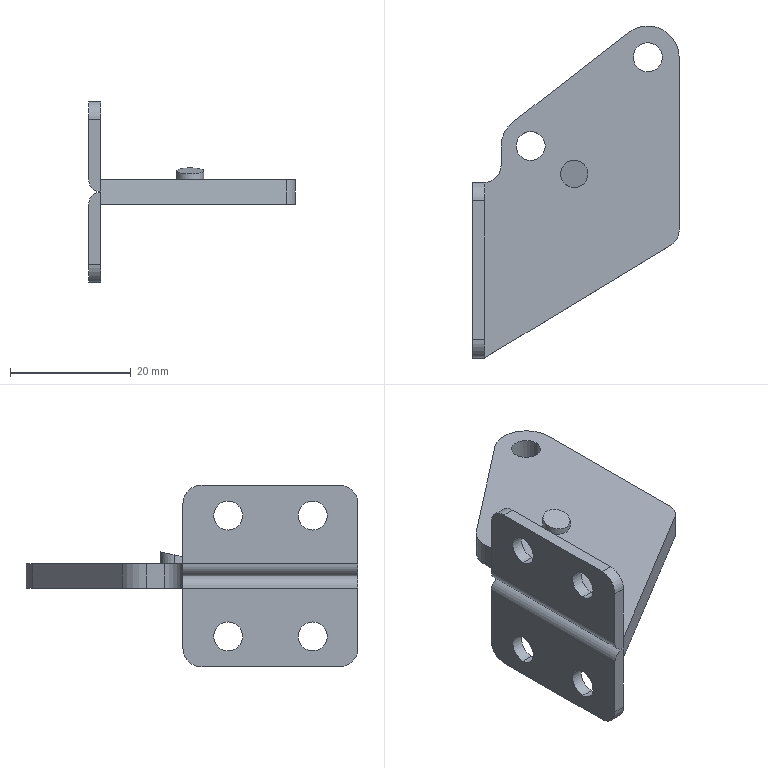Part | SolidWorks | features BaseBody 1 | 1 solid | 42 faces | box 34.2 x 55.001 x 30 mm | volume 6148 mm3 | cylinder 24 | plane 18 | commonest cylinder face diameters 4.8 x12 6 x5 4 x2 4.5 x2 6.004 x1 10 x1
STEP:
#1=CARTESIAN_POINT('',(31.4,49.8,-2.));
#2=VERTEX_POINT('',#1);
#3=CARTESIAN_POINT('',(26.6,49.8,-2.));
#4=VERTEX_POINT('',#3);
#5=CARTESIAN_POINT('',(29.,49.8,-2.));
#6=DIRECTION('',(0.,0.,-1.));
#7=DIRECTION('',(1.,0.,0.));
#8=AXIS2_PLACEMENT_3D('',#5,#6,#7);
#9=CIRCLE('',#8,2.4);
#10=EDGE_CURVE('',#2,#4,#9,.T.);
#11=ORIENTED_EDGE('',*,*,#10,.T.);
#12=CARTESIAN_POINT('',(26.6,49.8,2.));
#13=VERTEX_POINT('',#12);
#14=CARTESIAN_POINT('',(26.6,49.8,2.));
#15=DIRECTION('',(0.,0.,1.));
#16=VECTOR('',#15,1000.);
#17=LINE('',#14,#16);
#18=EDGE_CURVE('',#4,#13,#17,.T.);
#19=ORIENTED_EDGE('',*,*,#18,.T.);
#20=CARTESIAN_POINT('',(31.4,49.8,2.));
#21=VERTEX_POINT('',#20);
#22=CARTESIAN_POINT('',(29.,49.8,2.));
#23=DIRECTION('',(0.,0.,-1.));
#24=DIRECTION('',(1.,0.,0.));
#25=AXIS2_PLACEMENT_3D('',#22,#23,#24);
#26=CIRCLE('',#25,2.4);
#27=EDGE_CURVE('',#21,#13,#26,.T.);
#28=ORIENTED_EDGE('',*,*,#27,.F.);
#29=CARTESIAN_POINT('',(31.4,49.8,2.));
#30=DIRECTION('',(0.,0.,1.));
#31=VECTOR('',#30,1000.);
#32=LINE('',#29,#31);
#33=EDGE_CURVE('',#2,#21,#32,.T.);
#34=ORIENTED_EDGE('',*,*,#33,.F.);
#35=EDGE_LOOP('',(#11,#19,#28,#34));
#36=FACE_OUTER_BOUND('',#35,.T.);
#37=CARTESIAN_POINT('',(29.,49.8,2.));
#38=DIRECTION('',(0.,0.,1.));
#39=DIRECTION('',(1.,0.,0.));
#40=AXIS2_PLACEMENT_3D('',#37,#38,#39);
#41=CYLINDRICAL_SURFACE('',#40,2.4);
#42=ADVANCED_FACE('',(#36),#41,.F.);
#43=CARTESIAN_POINT('',(12.,35.1,-2.));
#44=VERTEX_POINT('',#43);
#45=CARTESIAN_POINT('',(7.2,35.1,-2.));
#46=VERTEX_POINT('',#45);
#47=CARTESIAN_POINT('',(9.6,35.1,-2.));
#48=DIRECTION('',(0.,0.,-1.));
#49=DIRECTION('',(1.,0.,0.));
#50=AXIS2_PLACEMENT_3D('',#47,#48,#49);
#51=CIRCLE('',#50,2.4);
#52=EDGE_CURVE('',#44,#46,#51,.T.);
#53=ORIENTED_EDGE('',*,*,#52,.T.);
#54=CARTESIAN_POINT('',(7.2,35.1,2.));
#55=VERTEX_POINT('',#54);
#56=CARTESIAN_POINT('',(7.2,35.1,2.));
#57=DIRECTION('',(0.,0.,1.));
#58=VECTOR('',#57,1000.);
#59=LINE('',#56,#58);
#60=EDGE_CURVE('',#46,#55,#59,.T.);
#61=ORIENTED_EDGE('',*,*,#60,.T.);
#62=CARTESIAN_POINT('',(12.,35.1,2.));
#63=VERTEX_POINT('',#62);
#64=CARTESIAN_POINT('',(9.6,35.1,2.));
#65=DIRECTION('',(0.,0.,-1.));
#66=DIRECTION('',(1.,0.,0.));
#67=AXIS2_PLACEMENT_3D('',#64,#65,#66);
#68=CIRCLE('',#67,2.4);
#69=EDGE_CURVE('',#63,#55,#68,.T.);
#70=ORIENTED_EDGE('',*,*,#69,.F.);
#71=CARTESIAN_POINT('',(12.,35.1,2.));
#72=DIRECTION('',(0.,0.,1.));
#73=VECTOR('',#72,1000.);
#74=LINE('',#71,#73);
#75=EDGE_CURVE('',#44,#63,#74,.T.);
#76=ORIENTED_EDGE('',*,*,#75,.F.);
#77=EDGE_LOOP('',(#53,#61,#70,#76));
#78=FACE_OUTER_BOUND('',#77,.T.);
#79=CARTESIAN_POINT('',(9.6,35.1,2.));
#80=DIRECTION('',(0.,0.,1.));
#81=DIRECTION('',(1.,0.,0.));
#82=AXIS2_PLACEMENT_3D('',#79,#80,#81);
#83=CYLINDRICAL_SURFACE('',#82,2.4);
#84=ADVANCED_FACE('',(#78),#83,.F.);
#85=CARTESIAN_POINT('',(0.,7.5,-7.6));
#86=VERTEX_POINT('',#85);
#87=CARTESIAN_POINT('',(0.,7.5,-12.4));
#88=VERTEX_POINT('',#87);
#89=CARTESIAN_POINT('',(0.,7.5,-10.));
#90=DIRECTION('',(1.,0.,0.));
#91=DIRECTION('',(0.,0.,-1.));
#92=AXIS2_PLACEMENT_3D('',#89,#90,#91);
#93=CIRCLE('',#92,2.4);
#94=EDGE_CURVE('',#86,#88,#93,.T.);
#95=ORIENTED_EDGE('',*,*,#94,.F.);
#96=CARTESIAN_POINT('',(2.,7.5,-7.6));
#97=VERTEX_POINT('',#96);
#98=CARTESIAN_POINT('',(2.,7.5,-7.6));
#99=DIRECTION('',(1.,0.,0.));
#100=VECTOR('',#99,1000.);
#101=LINE('',#98,#100);
#102=EDGE_CURVE('',#86,#97,#101,.T.);
#103=ORIENTED_EDGE('',*,*,#102,.T.);
#104=CARTESIAN_POINT('',(2.,7.5,-12.4));
#105=VERTEX_POINT('',#104);
#106=CARTESIAN_POINT('',(2.,7.5,-10.));
#107=DIRECTION('',(-1.,0.,0.));
#108=DIRECTION('',(0.,0.,-1.));
#109=AXIS2_PLACEMENT_3D('',#106,#107,#108);
#110=CIRCLE('',#109,2.4);
#111=EDGE_CURVE('',#105,#97,#110,.T.);
#112=ORIENTED_EDGE('',*,*,#111,.F.);
#113=CARTESIAN_POINT('',(2.,7.5,-12.4));
#114=DIRECTION('',(1.,0.,0.));
#115=VECTOR('',#114,1000.);
#116=LINE('',#113,#115);
#117=EDGE_CURVE('',#88,#105,#116,.T.);
#118=ORIENTED_EDGE('',*,*,#117,.F.);
#119=EDGE_LOOP('',(#95,#103,#112,#118));
#120=FACE_OUTER_BOUND('',#119,.T.);
#121=CARTESIAN_POINT('',(2.,7.5,-10.));
#122=DIRECTION('',(1.,0.,0.));
#123=DIRECTION('',(0.,0.,-1.));
#124=AXIS2_PLACEMENT_3D('',#121,#122,#123);
#125=CYLINDRICAL_SURFACE('',#124,2.4);
#126=ADVANCED_FACE('',(#120),#125,.F.);
#127=CARTESIAN_POINT('',(0.,21.5,-7.6));
#128=VERTEX_POINT('',#127);
#129=CARTESIAN_POINT('',(0.,21.5,-12.4));
#130=VERTEX_POINT('',#129);
#131=CARTESIAN_POINT('',(0.,21.5,-10.));
#132=DIRECTION('',(1.,0.,0.));
#133=DIRECTION('',(0.,0.,-1.));
#134=AXIS2_PLACEMENT_3D('',#131,#132,#133);
#135=CIRCLE('',#134,2.4);
#136=EDGE_CURVE('',#128,#130,#135,.T.);
#137=ORIENTED_EDGE('',*,*,#136,.F.);
#138=CARTESIAN_POINT('',(2.,21.5,-7.6));
#139=VERTEX_POINT('',#138);
#140=CARTESIAN_POINT('',(2.,21.5,-7.6));
#141=DIRECTION('',(1.,0.,0.));
#142=VECTOR('',#141,1000.);
#143=LINE('',#140,#142);
#144=EDGE_CURVE('',#128,#139,#143,.T.);
#145=ORIENTED_EDGE('',*,*,#144,.T.);
#146=CARTESIAN_POINT('',(2.,21.5,-12.4));
#147=VERTEX_POINT('',#146);
#148=CARTESIAN_POINT('',(2.,21.5,-10.));
#149=DIRECTION('',(-1.,0.,0.));
#150=DIRECTION('',(0.,0.,-1.));
#151=AXIS2_PLACEMENT_3D('',#148,#149,#150);
#152=CIRCLE('',#151,2.4);
#153=EDGE_CURVE('',#147,#139,#152,.T.);
#154=ORIENTED_EDGE('',*,*,#153,.F.);
#155=CARTESIAN_POINT('',(2.,21.5,-12.4));
#156=DIRECTION('',(1.,0.,0.));
#157=VECTOR('',#156,1000.);
#158=LINE('',#155,#157);
#159=EDGE_CURVE('',#130,#147,#158,.T.);
#160=ORIENTED_EDGE('',*,*,#159,.F.);
#161=EDGE_LOOP('',(#137,#145,#154,#160));
#162=FACE_OUTER_BOUND('',#161,.T.);
#163=CARTESIAN_POINT('',(2.,21.5,-10.));
#164=DIRECTION('',(1.,0.,0.));
#165=DIRECTION('',(0.,0.,-1.));
#166=AXIS2_PLACEMENT_3D('',#163,#164,#165);
#167=CYLINDRICAL_SURFACE('',#166,2.4);
#168=ADVANCED_FACE('',(#162),#167,.F.);
#169=CARTESIAN_POINT('',(14.55,30.472,2.));
#170=VERTEX_POINT('',#169);
#171=CARTESIAN_POINT('',(19.05,30.472,2.));
#172=VERTEX_POINT('',#171);
#173=CARTESIAN_POINT('',(16.8,30.472,2.));
#174=DIRECTION('',(0.,0.,-1.));
#175=DIRECTION('',(1.,0.,0.));
#176=AXIS2_PLACEMENT_3D('',#173,#174,#175);
#177=CIRCLE('',#176,2.25);
#178=EDGE_CURVE('',#170,#172,#177,.T.);
#179=ORIENTED_EDGE('',*,*,#178,.F.);
#180=CARTESIAN_POINT('',(14.55,30.472,3.5));
#181=VERTEX_POINT('',#180);
#182=CARTESIAN_POINT('',(14.55,30.472,4.));
#183=DIRECTION('',(0.,0.,1.));
#184=VECTOR('',#183,1000.);
#185=LINE('',#182,#184);
#186=EDGE_CURVE('',#170,#181,#185,.T.);
#187=ORIENTED_EDGE('',*,*,#186,.T.);
#188=CARTESIAN_POINT('',(19.05,30.472,3.5));
#189=VERTEX_POINT('',#188);
#190=CARTESIAN_POINT('',(14.55,30.472,3.5));
#191=CARTESIAN_POINT('',(14.55,34.972,4.5));
#192=CARTESIAN_POINT('',(19.05,34.972,4.5));
#193=CARTESIAN_POINT('',(19.05,30.472,3.5));
#194=(BOUNDED_CURVE()B_SPLINE_CURVE(3,(#190,#191,#192,#193),.UNSPECIFIED.,.F.,.F.)B_SPLINE_CURVE_WITH_KNOTS((4,4),(4.712,7.854),.UNSPECIFIED.)CURVE()GEOMETRIC_REPRESENTATION_ITEM()RATIONAL_B_SPLINE_CURVE((1.,0.3333,0.3333,1.))REPRESENTATION_ITEM(''));
#195=EDGE_CURVE('',#181,#189,#194,.T.);
#196=ORIENTED_EDGE('',*,*,#195,.T.);
#197=CARTESIAN_POINT('',(19.05,30.472,4.));
#198=DIRECTION('',(0.,0.,1.));
#199=VECTOR('',#198,1000.);
#200=LINE('',#197,#199);
#201=EDGE_CURVE('',#172,#189,#200,.T.);
#202=ORIENTED_EDGE('',*,*,#201,.F.);
#203=EDGE_LOOP('',(#179,#187,#196,#202));
#204=FACE_OUTER_BOUND('',#203,.T.);
#205=CARTESIAN_POINT('',(16.8,30.472,4.));
#206=DIRECTION('',(0.,0.,1.));
#207=DIRECTION('',(1.,0.,0.));
#208=AXIS2_PLACEMENT_3D('',#205,#206,#207);
#209=CYLINDRICAL_SURFACE('',#208,2.25);
#210=ADVANCED_FACE('',(#204),#209,.T.);
#211=CARTESIAN_POINT('',(0.,21.5,7.6));
#212=VERTEX_POINT('',#211);
#213=CARTESIAN_POINT('',(0.,21.5,12.4));
#214=VERTEX_POINT('',#213);
#215=CARTESIAN_POINT('',(0.,21.5,10.));
#216=DIRECTION('',(-1.,0.,0.));
#217=DIRECTION('',(0.,0.,-1.));
#218=AXIS2_PLACEMENT_3D('',#215,#216,#217);
#219=CIRCLE('',#218,2.4);
#220=EDGE_CURVE('',#212,#214,#219,.T.);
#221=ORIENTED_EDGE('',*,*,#220,.T.);
#222=CARTESIAN_POINT('',(2.,21.5,12.4));
#223=VERTEX_POINT('',#222);
#224=CARTESIAN_POINT('',(2.,21.5,12.4));
#225=DIRECTION('',(1.,0.,0.));
#226=VECTOR('',#225,1000.);
#227=LINE('',#224,#226);
#228=EDGE_CURVE('',#214,#223,#227,.T.);
#229=ORIENTED_EDGE('',*,*,#228,.T.);
#230=CARTESIAN_POINT('',(2.,21.5,7.6));
#231=VERTEX_POINT('',#230);
#232=CARTESIAN_POINT('',(2.,21.5,10.));
#233=DIRECTION('',(-1.,0.,0.));
#234=DIRECTION('',(0.,0.,-1.));
#235=AXIS2_PLACEMENT_3D('',#232,#233,#234);
#236=CIRCLE('',#235,2.4);
#237=EDGE_CURVE('',#231,#223,#236,.T.);
#238=ORIENTED_EDGE('',*,*,#237,.F.);
#239=CARTESIAN_POINT('',(2.,21.5,7.6));
#240=DIRECTION('',(1.,0.,0.));
#241=VECTOR('',#240,1000.);
#242=LINE('',#239,#241);
#243=EDGE_CURVE('',#212,#231,#242,.T.);
#244=ORIENTED_EDGE('',*,*,#243,.F.);
#245=EDGE_LOOP('',(#221,#229,#238,#244));
#246=FACE_OUTER_BOUND('',#245,.T.);
#247=CARTESIAN_POINT('',(2.,21.5,10.));
#248=DIRECTION('',(1.,0.,0.));
#249=DIRECTION('',(0.,0.,-1.));
#250=AXIS2_PLACEMENT_3D('',#247,#248,#249);
#251=CYLINDRICAL_SURFACE('',#250,2.4);
#252=ADVANCED_FACE('',(#246),#251,.F.);
#253=CARTESIAN_POINT('',(0.,7.5,7.6));
#254=VERTEX_POINT('',#253);
#255=CARTESIAN_POINT('',(0.,7.5,12.4));
#256=VERTEX_POINT('',#255);
#257=CARTESIAN_POINT('',(0.,7.5,10.));
#258=DIRECTION('',(-1.,0.,0.));
#259=DIRECTION('',(0.,0.,-1.));
#260=AXIS2_PLACEMENT_3D('',#257,#258,#259);
#261=CIRCLE('',#260,2.4);
#262=EDGE_CURVE('',#254,#256,#261,.T.);
#263=ORIENTED_EDGE('',*,*,#262,.T.);
#264=CARTESIAN_POINT('',(2.,7.5,12.4));
#265=VERTEX_POINT('',#264);
#266=CARTESIAN_POINT('',(2.,7.5,12.4));
#267=DIRECTION('',(1.,0.,0.));
#268=VECTOR('',#267,1000.);
#269=LINE('',#266,#268);
#270=EDGE_CURVE('',#256,#265,#269,.T.);
#271=ORIENTED_EDGE('',*,*,#270,.T.);
#272=CARTESIAN_POINT('',(2.,7.5,7.6));
#273=VERTEX_POINT('',#272);
#274=CARTESIAN_POINT('',(2.,7.5,10.));
#275=DIRECTION('',(-1.,0.,0.));
#276=DIRECTION('',(0.,0.,-1.));
#277=AXIS2_PLACEMENT_3D('',#274,#275,#276);
#278=CIRCLE('',#277,2.4);
#279=EDGE_CURVE('',#273,#265,#278,.T.);
#280=ORIENTED_EDGE('',*,*,#279,.F.);
#281=CARTESIAN_POINT('',(2.,7.5,7.6));
#282=DIRECTION('',(1.,0.,0.));
#283=VECTOR('',#282,1000.);
#284=LINE('',#281,#283);
#285=EDGE_CURVE('',#254,#273,#284,.T.);
#286=ORIENTED_EDGE('',*,*,#285,.F.);
#287=EDGE_LOOP('',(#263,#271,#280,#286));
#288=FACE_OUTER_BOUND('',#287,.T.);
#289=CARTESIAN_POINT('',(2.,7.5,10.));
#290=DIRECTION('',(1.,0.,0.));
#291=DIRECTION('',(0.,0.,-1.));
#292=AXIS2_PLACEMENT_3D('',#289,#290,#291);
#293=CYLINDRICAL_SURFACE('',#292,2.4);
#294=ADVANCED_FACE('',(#288),#293,.F.);
#295=CARTESIAN_POINT('',(4.7,32.,-2.));
#296=VERTEX_POINT('',#295);
#297=CARTESIAN_POINT('',(2.,29.015,-2.));
#298=VERTEX_POINT('',#297);
#299=CARTESIAN_POINT('',(1.698,32.002,-2.));
#300=DIRECTION('',(0.,0.,-1.));
#301=DIRECTION('',(1.,0.,0.));
#302=AXIS2_PLACEMENT_3D('',#299,#300,#301);
#303=CIRCLE('',#302,3.002);
#304=EDGE_CURVE('',#296,#298,#303,.T.);
#305=ORIENTED_EDGE('',*,*,#304,.F.);
#306=CARTESIAN_POINT('',(4.7,35.1,-2.));
#307=VERTEX_POINT('',#306);
#308=CARTESIAN_POINT('',(4.7,21.206,-2.));
#309=DIRECTION('',(0.,-1.,0.));
#310=VECTOR('',#309,1000.);
#311=LINE('',#308,#310);
#312=EDGE_CURVE('',#307,#296,#311,.T.);
#313=ORIENTED_EDGE('',*,*,#312,.F.);
#314=CARTESIAN_POINT('',(6.638,39.053,-2.));
#315=VERTEX_POINT('',#314);
#316=CARTESIAN_POINT('',(9.7,35.1,-2.));
#317=DIRECTION('',(0.,0.,1.));
#318=DIRECTION('',(1.,0.,0.));
#319=AXIS2_PLACEMENT_3D('',#316,#317,#318);
#320=CIRCLE('',#319,5.);
#321=EDGE_CURVE('',#315,#307,#320,.T.);
#322=ORIENTED_EDGE('',*,*,#321,.F.);
#323=CARTESIAN_POINT('',(25.815,53.911,-2.));
#324=VERTEX_POINT('',#323);
#325=CARTESIAN_POINT('',(25.815,53.911,-2.));
#326=DIRECTION('',(-0.7905,-0.6125,0.));
#327=VECTOR('',#326,1000.);
#328=LINE('',#325,#327);
#329=EDGE_CURVE('',#324,#315,#328,.T.);
#330=ORIENTED_EDGE('',*,*,#329,.F.);
#331=CARTESIAN_POINT('',(34.2,49.801,-2.));
#332=VERTEX_POINT('',#331);
#333=CARTESIAN_POINT('',(29.,49.801,-2.));
#334=DIRECTION('',(0.,0.,1.));
#335=DIRECTION('',(1.,0.,0.));
#336=AXIS2_PLACEMENT_3D('',#333,#334,#335);
#337=CIRCLE('',#336,5.2);
#338=EDGE_CURVE('',#332,#324,#337,.T.);
#339=ORIENTED_EDGE('',*,*,#338,.F.);
#340=CARTESIAN_POINT('',(34.2,21.206,-2.));
#341=VERTEX_POINT('',#340);
#342=CARTESIAN_POINT('',(34.2,21.206,-2.));
#343=DIRECTION('',(0.,1.,0.));
#344=VECTOR('',#343,1000.);
#345=LINE('',#342,#344);
#346=EDGE_CURVE('',#341,#332,#345,.T.);
#347=ORIENTED_EDGE('',*,*,#346,.F.);
#348=CARTESIAN_POINT('',(32.755,18.64,-2.));
#349=VERTEX_POINT('',#348);
#350=CARTESIAN_POINT('',(31.2,21.206,-2.));
#351=DIRECTION('',(0.,0.,1.));
#352=DIRECTION('',(1.,0.,0.));
#353=AXIS2_PLACEMENT_3D('',#350,#351,#352);
#354=CIRCLE('',#353,3.);
#355=EDGE_CURVE('',#349,#341,#354,.T.);
#356=ORIENTED_EDGE('',*,*,#355,.F.);
#357=CARTESIAN_POINT('',(2.,0.,-2.));
#358=VERTEX_POINT('',#357);
#359=CARTESIAN_POINT('',(2.,0.,-2.));
#360=DIRECTION('',(0.8552,0.5183,0.));
#361=VECTOR('',#360,1000.);
#362=LINE('',#359,#361);
#363=EDGE_CURVE('',#358,#349,#362,.T.);
#364=ORIENTED_EDGE('',*,*,#363,.F.);
#365=CARTESIAN_POINT('',(2.,29.,-2.));
#366=VERTEX_POINT('',#365);
#367=CARTESIAN_POINT('',(2.,21.206,-2.));
#368=DIRECTION('',(0.,-1.,0.));
#369=VECTOR('',#368,1000.);
#370=LINE('',#367,#369);
#371=EDGE_CURVE('',#366,#358,#370,.T.);
#372=ORIENTED_EDGE('',*,*,#371,.F.);
#373=CARTESIAN_POINT('',(2.,29.015,-2.));
#374=DIRECTION('',(0.,1.,0.));
#375=VECTOR('',#374,1000.);
#376=LINE('',#373,#375);
#377=EDGE_CURVE('',#366,#298,#376,.T.);
#378=ORIENTED_EDGE('',*,*,#377,.T.);
#379=EDGE_LOOP('',(#305,#313,#322,#330,#339,#347,#356,#364,#372,#378));
#380=FACE_OUTER_BOUND('',#379,.T.);
#381=ORIENTED_EDGE('',*,*,#10,.F.);
#382=CARTESIAN_POINT('',(29.,49.8,-2.));
#383=DIRECTION('',(0.,0.,-1.));
#384=DIRECTION('',(1.,0.,0.));
#385=AXIS2_PLACEMENT_3D('',#382,#383,#384);
#386=CIRCLE('',#385,2.4);
#387=EDGE_CURVE('',#4,#2,#386,.T.);
#388=ORIENTED_EDGE('',*,*,#387,.F.);
#389=EDGE_LOOP('',(#381,#388));
#390=FACE_BOUND('',#389,.T.);
#391=ORIENTED_EDGE('',*,*,#52,.F.);
#392=CARTESIAN_POINT('',(9.6,35.1,-2.));
#393=DIRECTION('',(0.,0.,-1.));
#394=DIRECTION('',(1.,0.,0.));
#395=AXIS2_PLACEMENT_3D('',#392,#393,#394);
#396=CIRCLE('',#395,2.4);
#397=EDGE_CURVE('',#46,#44,#396,.T.);
#398=ORIENTED_EDGE('',*,*,#397,.F.);
#399=EDGE_LOOP('',(#391,#398));
#400=FACE_BOUND('',#399,.T.);
#401=CARTESIAN_POINT('',(31.2,21.206,-2.));
#402=DIRECTION('',(0.,0.,1.));
#403=DIRECTION('',(1.,0.,0.));
#404=AXIS2_PLACEMENT_3D('',#401,#402,#403);
#405=PLANE('',#404);
#406=ADVANCED_FACE('',(#380,#390,#400),#405,.F.);
#407=CARTESIAN_POINT('',(2.,29.015,2.));
#408=VERTEX_POINT('',#407);
#409=CARTESIAN_POINT('',(2.,29.015,2.));
#410=DIRECTION('',(0.,0.,-1.));
#411=VECTOR('',#410,1000.);
#412=LINE('',#409,#411);
#413=EDGE_CURVE('',#408,#298,#412,.T.);
#414=ORIENTED_EDGE('',*,*,#413,.F.);
#415=CARTESIAN_POINT('',(4.7,32.,2.));
#416=VERTEX_POINT('',#415);
#417=CARTESIAN_POINT('',(1.698,32.002,2.));
#418=DIRECTION('',(0.,0.,-1.));
#419=DIRECTION('',(1.,0.,0.));
#420=AXIS2_PLACEMENT_3D('',#417,#418,#419);
#421=CIRCLE('',#420,3.002);
#422=EDGE_CURVE('',#416,#408,#421,.T.);
#423=ORIENTED_EDGE('',*,*,#422,.F.);
#424=CARTESIAN_POINT('',(4.7,32.,2.));
#425=DIRECTION('',(0.,0.,1.));
#426=VECTOR('',#425,1000.);
#427=LINE('',#424,#426);
#428=EDGE_CURVE('',#296,#416,#427,.T.);
#429=ORIENTED_EDGE('',*,*,#428,.F.);
#430=ORIENTED_EDGE('',*,*,#304,.T.);
#431=EDGE_LOOP('',(#414,#423,#429,#430));
#432=FACE_OUTER_BOUND('',#431,.T.);
#433=CARTESIAN_POINT('',(1.698,32.002,2.));
#434=DIRECTION('',(0.,0.,1.));
#435=DIRECTION('',(1.,0.,0.));
#436=AXIS2_PLACEMENT_3D('',#433,#434,#435);
#437=CYLINDRICAL_SURFACE('',#436,3.002);
#438=ADVANCED_FACE('',(#432),#437,.F.);
#439=ORIENTED_EDGE('',*,*,#428,.T.);
#440=CARTESIAN_POINT('',(4.7,35.1,2.));
#441=VERTEX_POINT('',#440);
#442=CARTESIAN_POINT('',(4.7,35.1,2.));
#443=DIRECTION('',(0.,-1.,0.));
#444=VECTOR('',#443,1000.);
#445=LINE('',#442,#444);
#446=EDGE_CURVE('',#441,#416,#445,.T.);
#447=ORIENTED_EDGE('',*,*,#446,.F.);
#448=CARTESIAN_POINT('',(4.7,35.1,2.));
#449=DIRECTION('',(0.,0.,1.));
#450=VECTOR('',#449,1000.);
#451=LINE('',#448,#450);
#452=EDGE_CURVE('',#307,#441,#451,.T.);
#453=ORIENTED_EDGE('',*,*,#452,.F.);
#454=ORIENTED_EDGE('',*,*,#312,.T.);
#455=EDGE_LOOP('',(#439,#447,#453,#454));
#456=FACE_OUTER_BOUND('',#455,.T.);
#457=CARTESIAN_POINT('',(4.7,35.1,2.));
#458=DIRECTION('',(1.,0.,0.));
#459=DIRECTION('',(0.,1.,0.));
#460=AXIS2_PLACEMENT_3D('',#457,#458,#459);
#461=PLANE('',#460);
#462=ADVANCED_FACE('',(#456),#461,.F.);
#463=CARTESIAN_POINT('',(6.638,39.053,2.));
#464=VERTEX_POINT('',#463);
#465=CARTESIAN_POINT('',(9.7,35.1,2.));
#466=DIRECTION('',(0.,0.,-1.));
#467=DIRECTION('',(1.,0.,0.));
#468=AXIS2_PLACEMENT_3D('',#465,#466,#467);
#469=CIRCLE('',#468,5.);
#470=EDGE_CURVE('',#441,#464,#469,.T.);
#471=ORIENTED_EDGE('',*,*,#470,.T.);
#472=CARTESIAN_POINT('',(6.638,39.053,2.));
#473=DIRECTION('',(0.,0.,-1.));
#474=VECTOR('',#473,1000.);
#475=LINE('',#472,#474);
#476=EDGE_CURVE('',#464,#315,#475,.T.);
#477=ORIENTED_EDGE('',*,*,#476,.T.);
#478=ORIENTED_EDGE('',*,*,#321,.T.);
#479=ORIENTED_EDGE('',*,*,#452,.T.);
#480=EDGE_LOOP('',(#471,#477,#478,#479));
#481=FACE_OUTER_BOUND('',#480,.T.);
#482=CARTESIAN_POINT('',(9.7,35.1,2.));
#483=DIRECTION('',(0.,0.,1.));
#484=DIRECTION('',(1.,0.,0.));
#485=AXIS2_PLACEMENT_3D('',#482,#483,#484);
#486=CYLINDRICAL_SURFACE('',#485,5.);
#487=ADVANCED_FACE('',(#481),#486,.T.);
#488=ORIENTED_EDGE('',*,*,#476,.F.);
#489=CARTESIAN_POINT('',(25.815,53.911,2.));
#490=VERTEX_POINT('',#489);
#491=CARTESIAN_POINT('',(25.815,53.911,2.));
#492=DIRECTION('',(-0.7905,-0.6125,0.));
#493=VECTOR('',#492,1000.);
#494=LINE('',#491,#493);
#495=EDGE_CURVE('',#490,#464,#494,.T.);
#496=ORIENTED_EDGE('',*,*,#495,.F.);
#497=CARTESIAN_POINT('',(25.815,53.911,2.));
#498=DIRECTION('',(0.,0.,1.));
#499=VECTOR('',#498,1000.);
#500=LINE('',#497,#499);
#501=EDGE_CURVE('',#324,#490,#500,.T.);
#502=ORIENTED_EDGE('',*,*,#501,.F.);
#503=ORIENTED_EDGE('',*,*,#329,.T.);
#504=EDGE_LOOP('',(#488,#496,#502,#503));
#505=FACE_OUTER_BOUND('',#504,.T.);
#506=CARTESIAN_POINT('',(25.815,53.911,2.));
#507=DIRECTION('',(0.6125,-0.7905,0.));
#508=DIRECTION('',(0.7905,0.6125,0.));
#509=AXIS2_PLACEMENT_3D('',#506,#507,#508);
#510=PLANE('',#509);
#511=ADVANCED_FACE('',(#505),#510,.F.);
#512=CARTESIAN_POINT('',(34.2,49.801,2.));
#513=VERTEX_POINT('',#512);
#514=CARTESIAN_POINT('',(29.,49.801,2.));
#515=DIRECTION('',(0.,0.,-1.));
#516=DIRECTION('',(1.,0.,0.));
#517=AXIS2_PLACEMENT_3D('',#514,#515,#516);
#518=CIRCLE('',#517,5.2);
#519=EDGE_CURVE('',#490,#513,#518,.T.);
#520=ORIENTED_EDGE('',*,*,#519,.T.);
#521=CARTESIAN_POINT('',(34.2,49.801,2.));
#522=DIRECTION('',(0.,0.,-1.));
#523=VECTOR('',#522,1000.);
#524=LINE('',#521,#523);
#525=EDGE_CURVE('',#513,#332,#524,.T.);
#526=ORIENTED_EDGE('',*,*,#525,.T.);
#527=ORIENTED_EDGE('',*,*,#338,.T.);
#528=ORIENTED_EDGE('',*,*,#501,.T.);
#529=EDGE_LOOP('',(#520,#526,#527,#528));
#530=FACE_OUTER_BOUND('',#529,.T.);
#531=CARTESIAN_POINT('',(29.,49.801,2.));
#532=DIRECTION('',(0.,0.,1.));
#533=DIRECTION('',(1.,0.,0.));
#534=AXIS2_PLACEMENT_3D('',#531,#532,#533);
#535=CYLINDRICAL_SURFACE('',#534,5.2);
#536=ADVANCED_FACE('',(#530),#535,.T.);
#537=ORIENTED_EDGE('',*,*,#525,.F.);
#538=CARTESIAN_POINT('',(34.2,21.206,2.));
#539=VERTEX_POINT('',#538);
#540=CARTESIAN_POINT('',(34.2,21.206,2.));
#541=DIRECTION('',(0.,1.,0.));
#542=VECTOR('',#541,1000.);
#543=LINE('',#540,#542);
#544=EDGE_CURVE('',#539,#513,#543,.T.);
#545=ORIENTED_EDGE('',*,*,#544,.F.);
#546=CARTESIAN_POINT('',(34.2,21.206,2.));
#547=DIRECTION('',(0.,0.,1.));
#548=VECTOR('',#547,1000.);
#549=LINE('',#546,#548);
#550=EDGE_CURVE('',#341,#539,#549,.T.);
#551=ORIENTED_EDGE('',*,*,#550,.F.);
#552=ORIENTED_EDGE('',*,*,#346,.T.);
#553=EDGE_LOOP('',(#537,#545,#551,#552));
#554=FACE_OUTER_BOUND('',#553,.T.);
#555=CARTESIAN_POINT('',(34.2,21.206,2.));
#556=DIRECTION('',(-1.,0.,0.));
#557=DIRECTION('',(0.,0.,1.));
#558=AXIS2_PLACEMENT_3D('',#555,#556,#557);
#559=PLANE('',#558);
#560=ADVANCED_FACE('',(#554),#559,.F.);
#561=CARTESIAN_POINT('',(32.755,18.64,2.));
#562=VERTEX_POINT('',#561);
#563=CARTESIAN_POINT('',(31.2,21.206,2.));
#564=DIRECTION('',(0.,0.,-1.));
#565=DIRECTION('',(1.,0.,0.));
#566=AXIS2_PLACEMENT_3D('',#563,#564,#565);
#567=CIRCLE('',#566,3.);
#568=EDGE_CURVE('',#539,#562,#567,.T.);
#569=ORIENTED_EDGE('',*,*,#568,.T.);
#570=CARTESIAN_POINT('',(32.755,18.64,2.));
#571=DIRECTION('',(0.,0.,-1.));
#572=VECTOR('',#571,1000.);
#573=LINE('',#570,#572);
#574=EDGE_CURVE('',#562,#349,#573,.T.);
#575=ORIENTED_EDGE('',*,*,#574,.T.);
#576=ORIENTED_EDGE('',*,*,#355,.T.);
#577=ORIENTED_EDGE('',*,*,#550,.T.);
#578=EDGE_LOOP('',(#569,#575,#576,#577));
#579=FACE_OUTER_BOUND('',#578,.T.);
#580=CARTESIAN_POINT('',(31.2,21.206,2.));
#581=DIRECTION('',(0.,0.,1.));
#582=DIRECTION('',(1.,0.,0.));
#583=AXIS2_PLACEMENT_3D('',#580,#581,#582);
#584=CYLINDRICAL_SURFACE('',#583,3.);
#585=ADVANCED_FACE('',(#579),#584,.T.);
#586=ORIENTED_EDGE('',*,*,#574,.F.);
#587=CARTESIAN_POINT('',(2.,0.,2.));
#588=VERTEX_POINT('',#587);
#589=CARTESIAN_POINT('',(2.,0.,2.));
#590=DIRECTION('',(0.8552,0.5183,0.));
#591=VECTOR('',#590,1000.);
#592=LINE('',#589,#591);
#593=EDGE_CURVE('',#588,#562,#592,.T.);
#594=ORIENTED_EDGE('',*,*,#593,.F.);
#595=CARTESIAN_POINT('',(2.,0.,0.));
#596=VERTEX_POINT('',#595);
#597=CARTESIAN_POINT('',(2.,0.,2.));
#598=DIRECTION('',(0.,0.,1.));
#599=VECTOR('',#598,1000.);
#600=LINE('',#597,#599);
#601=EDGE_CURVE('',#596,#588,#600,.T.);
#602=ORIENTED_EDGE('',*,*,#601,.F.);
#603=CARTESIAN_POINT('',(2.,0.,2.));
#604=DIRECTION('',(0.,0.,1.));
#605=VECTOR('',#604,1000.);
#606=LINE('',#603,#605);
#607=EDGE_CURVE('',#358,#596,#606,.T.);
#608=ORIENTED_EDGE('',*,*,#607,.F.);
#609=ORIENTED_EDGE('',*,*,#363,.T.);
#610=EDGE_LOOP('',(#586,#594,#602,#608,#609));
#611=FACE_OUTER_BOUND('',#610,.T.);
#612=CARTESIAN_POINT('',(2.,0.,2.));
#613=DIRECTION('',(-0.5183,0.8552,0.));
#614=DIRECTION('',(-0.8552,-0.5183,0.));
#615=AXIS2_PLACEMENT_3D('',#612,#613,#614);
#616=PLANE('',#615);
#617=ADVANCED_FACE('',(#611),#616,.F.);
#618=CARTESIAN_POINT('',(2.,3.,-15.));
#619=VERTEX_POINT('',#618);
#620=CARTESIAN_POINT('',(2.,26.,-15.));
#621=VERTEX_POINT('',#620);
#622=CARTESIAN_POINT('',(2.,26.,-15.));
#623=DIRECTION('',(0.,1.,0.));
#624=VECTOR('',#623,1000.);
#625=LINE('',#622,#624);
#626=EDGE_CURVE('',#619,#621,#625,.T.);
#627=ORIENTED_EDGE('',*,*,#626,.T.);
#628=CARTESIAN_POINT('',(2.,29.,-12.));
#629=VERTEX_POINT('',#628);
#630=CARTESIAN_POINT('',(2.,26.,-12.));
#631=DIRECTION('',(1.,0.,0.));
#632=DIRECTION('',(0.,0.,-1.));
#633=AXIS2_PLACEMENT_3D('',#630,#631,#632);
#634=CIRCLE('',#633,3.);
#635=EDGE_CURVE('',#621,#629,#634,.T.);
#636=ORIENTED_EDGE('',*,*,#635,.T.);
#637=CARTESIAN_POINT('',(2.,29.,12.));
#638=DIRECTION('',(0.,0.,1.));
#639=VECTOR('',#638,1000.);
#640=LINE('',#637,#639);
#641=EDGE_CURVE('',#629,#366,#640,.T.);
#642=ORIENTED_EDGE('',*,*,#641,.T.);
#643=ORIENTED_EDGE('',*,*,#371,.T.);
#644=CARTESIAN_POINT('',(2.,0.,-12.));
#645=VERTEX_POINT('',#644);
#646=CARTESIAN_POINT('',(2.,0.,12.));
#647=DIRECTION('',(0.,0.,-1.));
#648=VECTOR('',#647,1000.);
#649=LINE('',#646,#648);
#650=EDGE_CURVE('',#358,#645,#649,.T.);
#651=ORIENTED_EDGE('',*,*,#650,.T.);
#652=CARTESIAN_POINT('',(2.,3.,-12.));
#653=DIRECTION('',(1.,0.,0.));
#654=DIRECTION('',(0.,0.,-1.));
#655=AXIS2_PLACEMENT_3D('',#652,#653,#654);
#656=CIRCLE('',#655,3.);
#657=EDGE_CURVE('',#645,#619,#656,.T.);
#658=ORIENTED_EDGE('',*,*,#657,.T.);
#659=EDGE_LOOP('',(#627,#636,#642,#643,#651,#658));
#660=FACE_OUTER_BOUND('',#659,.T.);
#661=ORIENTED_EDGE('',*,*,#111,.T.);
#662=CARTESIAN_POINT('',(2.,7.5,-10.));
#663=DIRECTION('',(-1.,0.,0.));
#664=DIRECTION('',(0.,0.,-1.));
#665=AXIS2_PLACEMENT_3D('',#662,#663,#664);
#666=CIRCLE('',#665,2.4);
#667=EDGE_CURVE('',#97,#105,#666,.T.);
#668=ORIENTED_EDGE('',*,*,#667,.T.);
#669=EDGE_LOOP('',(#661,#668));
#670=FACE_BOUND('',#669,.T.);
#671=ORIENTED_EDGE('',*,*,#153,.T.);
#672=CARTESIAN_POINT('',(2.,21.5,-10.));
#673=DIRECTION('',(-1.,0.,0.));
#674=DIRECTION('',(0.,0.,-1.));
#675=AXIS2_PLACEMENT_3D('',#672,#673,#674);
#676=CIRCLE('',#675,2.4);
#677=EDGE_CURVE('',#139,#147,#676,.T.);
#678=ORIENTED_EDGE('',*,*,#677,.T.);
#679=EDGE_LOOP('',(#671,#678));
#680=FACE_BOUND('',#679,.T.);
#681=CARTESIAN_POINT('',(2.,26.,12.));
#682=DIRECTION('',(1.,0.,0.));
#683=DIRECTION('',(0.,0.,-1.));
#684=AXIS2_PLACEMENT_3D('',#681,#682,#683);
#685=PLANE('',#684);
#686=ADVANCED_FACE('',(#660,#670,#680),#685,.T.);
#687=ORIENTED_EDGE('',*,*,#18,.F.);
#688=ORIENTED_EDGE('',*,*,#387,.T.);
#689=ORIENTED_EDGE('',*,*,#33,.T.);
#690=CARTESIAN_POINT('',(29.,49.8,2.));
#691=DIRECTION('',(0.,0.,-1.));
#692=DIRECTION('',(1.,0.,0.));
#693=AXIS2_PLACEMENT_3D('',#690,#691,#692);
#694=CIRCLE('',#693,2.4);
#695=EDGE_CURVE('',#13,#21,#694,.T.);
#696=ORIENTED_EDGE('',*,*,#695,.F.);
#697=EDGE_LOOP('',(#687,#688,#689,#696));
#698=FACE_OUTER_BOUND('',#697,.T.);
#699=CARTESIAN_POINT('',(29.,49.8,2.));
#700=DIRECTION('',(0.,0.,1.));
#701=DIRECTION('',(1.,0.,0.));
#702=AXIS2_PLACEMENT_3D('',#699,#700,#701);
#703=CYLINDRICAL_SURFACE('',#702,2.4);
#704=ADVANCED_FACE('',(#698),#703,.F.);
#705=ORIENTED_EDGE('',*,*,#60,.F.);
#706=ORIENTED_EDGE('',*,*,#397,.T.);
#707=ORIENTED_EDGE('',*,*,#75,.T.);
#708=CARTESIAN_POINT('',(9.6,35.1,2.));
#709=DIRECTION('',(0.,0.,-1.));
#710=DIRECTION('',(1.,0.,0.));
#711=AXIS2_PLACEMENT_3D('',#708,#709,#710);
#712=CIRCLE('',#711,2.4);
#713=EDGE_CURVE('',#55,#63,#712,.T.);
#714=ORIENTED_EDGE('',*,*,#713,.F.);
#715=EDGE_LOOP('',(#705,#706,#707,#714));
#716=FACE_OUTER_BOUND('',#715,.T.);
#717=CARTESIAN_POINT('',(9.6,35.1,2.));
#718=DIRECTION('',(0.,0.,1.));
#719=DIRECTION('',(1.,0.,0.));
#720=AXIS2_PLACEMENT_3D('',#717,#718,#719);
#721=CYLINDRICAL_SURFACE('',#720,2.4);
#722=ADVANCED_FACE('',(#716),#721,.F.);
#723=CARTESIAN_POINT('',(2.,29.,2.));
#724=VERTEX_POINT('',#723);
#725=CARTESIAN_POINT('',(2.,29.,0.));
#726=VERTEX_POINT('',#725);
#727=CARTESIAN_POINT('',(2.,29.,2.));
#728=DIRECTION('',(0.,0.,-1.));
#729=VECTOR('',#728,1000.);
#730=LINE('',#727,#729);
#731=EDGE_CURVE('',#724,#726,#730,.T.);
#732=ORIENTED_EDGE('',*,*,#731,.F.);
#733=CARTESIAN_POINT('',(2.,29.015,2.));
#734=DIRECTION('',(0.,-1.,0.));
#735=VECTOR('',#734,1000.);
#736=LINE('',#733,#735);
#737=EDGE_CURVE('',#408,#724,#736,.T.);
#738=ORIENTED_EDGE('',*,*,#737,.F.);
#739=ORIENTED_EDGE('',*,*,#413,.T.);
#740=ORIENTED_EDGE('',*,*,#377,.F.);
#741=CARTESIAN_POINT('',(2.,29.,2.));
#742=DIRECTION('',(0.,0.,-1.));
#743=VECTOR('',#742,1000.);
#744=LINE('',#741,#743);
#745=EDGE_CURVE('',#726,#366,#744,.T.);
#746=ORIENTED_EDGE('',*,*,#745,.F.);
#747=EDGE_LOOP('',(#732,#738,#739,#740,#746));
#748=FACE_OUTER_BOUND('',#747,.T.);
#749=CARTESIAN_POINT('',(2.,29.015,2.));
#750=DIRECTION('',(1.,0.,0.));
#751=DIRECTION('',(0.,0.,-1.));
#752=AXIS2_PLACEMENT_3D('',#749,#750,#751);
#753=PLANE('',#752);
#754=ADVANCED_FACE('',(#748),#753,.F.);
#755=ORIENTED_EDGE('',*,*,#446,.T.);
#756=ORIENTED_EDGE('',*,*,#422,.T.);
#757=ORIENTED_EDGE('',*,*,#737,.T.);
#758=CARTESIAN_POINT('',(2.,21.206,2.));
#759=DIRECTION('',(0.,-1.,0.));
#760=VECTOR('',#759,1000.);
#761=LINE('',#758,#760);
#762=EDGE_CURVE('',#724,#588,#761,.T.);
#763=ORIENTED_EDGE('',*,*,#762,.T.);
#764=ORIENTED_EDGE('',*,*,#593,.T.);
#765=ORIENTED_EDGE('',*,*,#568,.F.);
#766=ORIENTED_EDGE('',*,*,#544,.T.);
#767=ORIENTED_EDGE('',*,*,#519,.F.);
#768=ORIENTED_EDGE('',*,*,#495,.T.);
#769=ORIENTED_EDGE('',*,*,#470,.F.);
#770=EDGE_LOOP('',(#755,#756,#757,#763,#764,#765,#766,#767,#768,#769));
#771=FACE_OUTER_BOUND('',#770,.T.);
#772=ORIENTED_EDGE('',*,*,#27,.T.);
#773=ORIENTED_EDGE('',*,*,#695,.T.);
#774=EDGE_LOOP('',(#772,#773));
#775=FACE_BOUND('',#774,.T.);
#776=ORIENTED_EDGE('',*,*,#69,.T.);
#777=ORIENTED_EDGE('',*,*,#713,.T.);
#778=EDGE_LOOP('',(#776,#777));
#779=FACE_BOUND('',#778,.T.);
#780=CARTESIAN_POINT('',(16.8,30.472,2.));
#781=DIRECTION('',(0.,0.,-1.));
#782=DIRECTION('',(1.,0.,0.));
#783=AXIS2_PLACEMENT_3D('',#780,#781,#782);
#784=CIRCLE('',#783,2.25);
#785=EDGE_CURVE('',#172,#170,#784,.T.);
#786=ORIENTED_EDGE('',*,*,#785,.T.);
#787=ORIENTED_EDGE('',*,*,#178,.T.);
#788=EDGE_LOOP('',(#786,#787));
#789=FACE_BOUND('',#788,.T.);
#790=CARTESIAN_POINT('',(31.2,21.206,2.));
#791=DIRECTION('',(0.,0.,1.));
#792=DIRECTION('',(1.,0.,0.));
#793=AXIS2_PLACEMENT_3D('',#790,#791,#792);
#794=PLANE('',#793);
#795=ADVANCED_FACE('',(#771,#775,#779,#789),#794,.T.);
#796=CARTESIAN_POINT('',(0.,0.,2.));
#797=VERTEX_POINT('',#796);
#798=CARTESIAN_POINT('',(2.,0.,2.));
#799=DIRECTION('',(0.,1.,0.));
#800=DIRECTION('',(0.,0.,1.));
#801=AXIS2_PLACEMENT_3D('',#798,#799,#800);
#802=CIRCLE('',#801,2.);
#803=EDGE_CURVE('',#596,#797,#802,.T.);
#804=ORIENTED_EDGE('',*,*,#803,.F.);
#805=ORIENTED_EDGE('',*,*,#601,.T.);
#806=CARTESIAN_POINT('',(2.,0.,12.));
#807=VERTEX_POINT('',#806);
#808=CARTESIAN_POINT('',(2.,0.,12.));
#809=DIRECTION('',(0.,0.,-1.));
#810=VECTOR('',#809,1000.);
#811=LINE('',#808,#810);
#812=EDGE_CURVE('',#807,#588,#811,.T.);
#813=ORIENTED_EDGE('',*,*,#812,.F.);
#814=CARTESIAN_POINT('',(0.,0.,12.));
#815=VERTEX_POINT('',#814);
#816=CARTESIAN_POINT('',(2.,0.,12.));
#817=DIRECTION('',(1.,0.,0.));
#818=VECTOR('',#817,1000.);
#819=LINE('',#816,#818);
#820=EDGE_CURVE('',#815,#807,#819,.T.);
#821=ORIENTED_EDGE('',*,*,#820,.F.);
#822=CARTESIAN_POINT('',(0.,0.,12.));
#823=DIRECTION('',(0.,0.,1.));
#824=VECTOR('',#823,1000.);
#825=LINE('',#822,#824);
#826=EDGE_CURVE('',#797,#815,#825,.T.);
#827=ORIENTED_EDGE('',*,*,#826,.F.);
#828=EDGE_LOOP('',(#804,#805,#813,#821,#827));
#829=FACE_OUTER_BOUND('',#828,.T.);
#830=CARTESIAN_POINT('',(2.,0.,12.));
#831=DIRECTION('',(0.,1.,0.));
#832=DIRECTION('',(0.,0.,1.));
#833=AXIS2_PLACEMENT_3D('',#830,#831,#832);
#834=PLANE('',#833);
#835=ADVANCED_FACE('',(#829),#834,.F.);
#836=CARTESIAN_POINT('',(0.,0.,-2.));
#837=VERTEX_POINT('',#836);
#838=CARTESIAN_POINT('',(2.,0.,-2.));
#839=DIRECTION('',(0.,1.,0.));
#840=DIRECTION('',(0.,0.,1.));
#841=AXIS2_PLACEMENT_3D('',#838,#839,#840);
#842=CIRCLE('',#841,2.);
#843=EDGE_CURVE('',#837,#596,#842,.T.);
#844=ORIENTED_EDGE('',*,*,#843,.F.);
#845=CARTESIAN_POINT('',(0.,0.,-12.));
#846=VERTEX_POINT('',#845);
#847=CARTESIAN_POINT('',(0.,0.,12.));
#848=DIRECTION('',(0.,0.,1.));
#849=VECTOR('',#848,1000.);
#850=LINE('',#847,#849);
#851=EDGE_CURVE('',#846,#837,#850,.T.);
#852=ORIENTED_EDGE('',*,*,#851,.F.);
#853=CARTESIAN_POINT('',(2.,0.,-12.));
#854=DIRECTION('',(-1.,0.,0.));
#855=VECTOR('',#854,1000.);
#856=LINE('',#853,#855);
#857=EDGE_CURVE('',#645,#846,#856,.T.);
#858=ORIENTED_EDGE('',*,*,#857,.F.);
#859=ORIENTED_EDGE('',*,*,#650,.F.);
#860=ORIENTED_EDGE('',*,*,#607,.T.);
#861=EDGE_LOOP('',(#844,#852,#858,#859,#860));
#862=FACE_OUTER_BOUND('',#861,.T.);
#863=CARTESIAN_POINT('',(2.,0.,12.));
#864=DIRECTION('',(0.,1.,0.));
#865=DIRECTION('',(0.,0.,1.));
#866=AXIS2_PLACEMENT_3D('',#863,#864,#865);
#867=PLANE('',#866);
#868=ADVANCED_FACE('',(#862),#867,.F.);
#869=ORIENTED_EDGE('',*,*,#635,.F.);
#870=CARTESIAN_POINT('',(0.,26.,-15.));
#871=VERTEX_POINT('',#870);
#872=CARTESIAN_POINT('',(2.,26.,-15.));
#873=DIRECTION('',(-1.,0.,0.));
#874=VECTOR('',#873,1000.);
#875=LINE('',#872,#874);
#876=EDGE_CURVE('',#621,#871,#875,.T.);
#877=ORIENTED_EDGE('',*,*,#876,.T.);
#878=CARTESIAN_POINT('',(0.,29.,-12.));
#879=VERTEX_POINT('',#878);
#880=CARTESIAN_POINT('',(0.,26.,-12.));
#881=DIRECTION('',(1.,0.,0.));
#882=DIRECTION('',(0.,0.,-1.));
#883=AXIS2_PLACEMENT_3D('',#880,#881,#882);
#884=CIRCLE('',#883,3.);
#885=EDGE_CURVE('',#871,#879,#884,.T.);
#886=ORIENTED_EDGE('',*,*,#885,.T.);
#887=CARTESIAN_POINT('',(2.,29.,-12.));
#888=DIRECTION('',(1.,0.,0.));
#889=VECTOR('',#888,1000.);
#890=LINE('',#887,#889);
#891=EDGE_CURVE('',#879,#629,#890,.T.);
#892=ORIENTED_EDGE('',*,*,#891,.T.);
#893=EDGE_LOOP('',(#869,#877,#886,#892));
#894=FACE_OUTER_BOUND('',#893,.T.);
#895=CARTESIAN_POINT('',(2.,26.,-12.));
#896=DIRECTION('',(1.,0.,0.));
#897=DIRECTION('',(0.,0.,-1.));
#898=AXIS2_PLACEMENT_3D('',#895,#896,#897);
#899=CYLINDRICAL_SURFACE('',#898,3.);
#900=ADVANCED_FACE('',(#894),#899,.T.);
#901=ORIENTED_EDGE('',*,*,#876,.F.);
#902=ORIENTED_EDGE('',*,*,#626,.F.);
#903=CARTESIAN_POINT('',(0.,3.,-15.));
#904=VERTEX_POINT('',#903);
#905=CARTESIAN_POINT('',(2.,3.,-15.));
#906=DIRECTION('',(1.,0.,0.));
#907=VECTOR('',#906,1000.);
#908=LINE('',#905,#907);
#909=EDGE_CURVE('',#904,#619,#908,.T.);
#910=ORIENTED_EDGE('',*,*,#909,.F.);
#911=CARTESIAN_POINT('',(0.,3.,-15.));
#912=DIRECTION('',(0.,-1.,0.));
#913=VECTOR('',#912,1000.);
#914=LINE('',#911,#913);
#915=EDGE_CURVE('',#871,#904,#914,.T.);
#916=ORIENTED_EDGE('',*,*,#915,.F.);
#917=EDGE_LOOP('',(#901,#902,#910,#916));
#918=FACE_OUTER_BOUND('',#917,.T.);
#919=CARTESIAN_POINT('',(2.,3.,-15.));
#920=DIRECTION('',(0.,0.,1.));
#921=DIRECTION('',(1.,0.,0.));
#922=AXIS2_PLACEMENT_3D('',#919,#920,#921);
#923=PLANE('',#922);
#924=ADVANCED_FACE('',(#918),#923,.F.);
#925=ORIENTED_EDGE('',*,*,#657,.F.);
#926=ORIENTED_EDGE('',*,*,#857,.T.);
#927=CARTESIAN_POINT('',(0.,3.,-12.));
#928=DIRECTION('',(1.,0.,0.));
#929=DIRECTION('',(0.,0.,-1.));
#930=AXIS2_PLACEMENT_3D('',#927,#928,#929);
#931=CIRCLE('',#930,3.);
#932=EDGE_CURVE('',#846,#904,#931,.T.);
#933=ORIENTED_EDGE('',*,*,#932,.T.);
#934=ORIENTED_EDGE('',*,*,#909,.T.);
#935=EDGE_LOOP('',(#925,#926,#933,#934));
#936=FACE_OUTER_BOUND('',#935,.T.);
#937=CARTESIAN_POINT('',(2.,3.,-12.));
#938=DIRECTION('',(1.,0.,0.));
#939=DIRECTION('',(0.,0.,-1.));
#940=AXIS2_PLACEMENT_3D('',#937,#938,#939);
#941=CYLINDRICAL_SURFACE('',#940,3.);
#942=ADVANCED_FACE('',(#936),#941,.T.);
#943=CARTESIAN_POINT('',(0.,29.,-2.));
#944=VERTEX_POINT('',#943);
#945=CARTESIAN_POINT('',(2.,29.,-2.));
#946=DIRECTION('',(0.,-1.,0.));
#947=DIRECTION('',(0.,0.,1.));
#948=AXIS2_PLACEMENT_3D('',#945,#946,#947);
#949=CIRCLE('',#948,2.);
#950=EDGE_CURVE('',#726,#944,#949,.T.);
#951=ORIENTED_EDGE('',*,*,#950,.F.);
#952=ORIENTED_EDGE('',*,*,#745,.T.);
#953=ORIENTED_EDGE('',*,*,#641,.F.);
#954=ORIENTED_EDGE('',*,*,#891,.F.);
#955=CARTESIAN_POINT('',(0.,29.,-12.));
#956=DIRECTION('',(0.,0.,-1.));
#957=VECTOR('',#956,1000.);
#958=LINE('',#955,#957);
#959=EDGE_CURVE('',#944,#879,#958,.T.);
#960=ORIENTED_EDGE('',*,*,#959,.F.);
#961=EDGE_LOOP('',(#951,#952,#953,#954,#960));
#962=FACE_OUTER_BOUND('',#961,.T.);
#963=CARTESIAN_POINT('',(2.,29.,-12.));
#964=DIRECTION('',(0.,-1.,0.));
#965=DIRECTION('',(0.,0.,-1.));
#966=AXIS2_PLACEMENT_3D('',#963,#964,#965);
#967=PLANE('',#966);
#968=ADVANCED_FACE('',(#962),#967,.F.);
#969=ORIENTED_EDGE('',*,*,#102,.F.);
#970=CARTESIAN_POINT('',(0.,7.5,-10.));
#971=DIRECTION('',(1.,0.,0.));
#972=DIRECTION('',(0.,0.,-1.));
#973=AXIS2_PLACEMENT_3D('',#970,#971,#972);
#974=CIRCLE('',#973,2.4);
#975=EDGE_CURVE('',#88,#86,#974,.T.);
#976=ORIENTED_EDGE('',*,*,#975,.F.);
#977=ORIENTED_EDGE('',*,*,#117,.T.);
#978=ORIENTED_EDGE('',*,*,#667,.F.);
#979=EDGE_LOOP('',(#969,#976,#977,#978));
#980=FACE_OUTER_BOUND('',#979,.T.);
#981=CARTESIAN_POINT('',(2.,7.5,-10.));
#982=DIRECTION('',(1.,0.,0.));
#983=DIRECTION('',(0.,0.,-1.));
#984=AXIS2_PLACEMENT_3D('',#981,#982,#983);
#985=CYLINDRICAL_SURFACE('',#984,2.4);
#986=ADVANCED_FACE('',(#980),#985,.F.);
#987=ORIENTED_EDGE('',*,*,#144,.F.);
#988=CARTESIAN_POINT('',(0.,21.5,-10.));
#989=DIRECTION('',(1.,0.,0.));
#990=DIRECTION('',(0.,0.,-1.));
#991=AXIS2_PLACEMENT_3D('',#988,#989,#990);
#992=CIRCLE('',#991,2.4);
#993=EDGE_CURVE('',#130,#128,#992,.T.);
#994=ORIENTED_EDGE('',*,*,#993,.F.);
#995=ORIENTED_EDGE('',*,*,#159,.T.);
#996=ORIENTED_EDGE('',*,*,#677,.F.);
#997=EDGE_LOOP('',(#987,#994,#995,#996));
#998=FACE_OUTER_BOUND('',#997,.T.);
#999=CARTESIAN_POINT('',(2.,21.5,-10.));
#1000=DIRECTION('',(1.,0.,0.));
#1001=DIRECTION('',(0.,0.,-1.));
#1002=AXIS2_PLACEMENT_3D('',#999,#1000,#1001);
#1003=CYLINDRICAL_SURFACE('',#1002,2.4);
#1004=ADVANCED_FACE('',(#998),#1003,.F.);
#1005=CARTESIAN_POINT('',(0.,29.,2.));
#1006=VERTEX_POINT('',#1005);
#1007=CARTESIAN_POINT('',(2.,29.,2.));
#1008=DIRECTION('',(0.,-1.,0.));
#1009=DIRECTION('',(0.,0.,1.));
#1010=AXIS2_PLACEMENT_3D('',#1007,#1008,#1009);
#1011=CIRCLE('',#1010,2.);
#1012=EDGE_CURVE('',#1006,#726,#1011,.T.);
#1013=ORIENTED_EDGE('',*,*,#1012,.F.);
#1014=CARTESIAN_POINT('',(0.,29.,12.));
#1015=VERTEX_POINT('',#1014);
#1016=CARTESIAN_POINT('',(0.,29.,-12.));
#1017=DIRECTION('',(0.,0.,-1.));
#1018=VECTOR('',#1017,1000.);
#1019=LINE('',#1016,#1018);
#1020=EDGE_CURVE('',#1015,#1006,#1019,.T.);
#1021=ORIENTED_EDGE('',*,*,#1020,.F.);
#1022=CARTESIAN_POINT('',(2.,29.,12.));
#1023=VERTEX_POINT('',#1022);
#1024=CARTESIAN_POINT('',(2.,29.,12.));
#1025=DIRECTION('',(-1.,0.,0.));
#1026=VECTOR('',#1025,1000.);
#1027=LINE('',#1024,#1026);
#1028=EDGE_CURVE('',#1023,#1015,#1027,.T.);
#1029=ORIENTED_EDGE('',*,*,#1028,.F.);
#1030=CARTESIAN_POINT('',(2.,29.,-12.));
#1031=DIRECTION('',(0.,0.,1.));
#1032=VECTOR('',#1031,1000.);
#1033=LINE('',#1030,#1032);
#1034=EDGE_CURVE('',#724,#1023,#1033,.T.);
#1035=ORIENTED_EDGE('',*,*,#1034,.F.);
#1036=ORIENTED_EDGE('',*,*,#731,.T.);
#1037=EDGE_LOOP('',(#1013,#1021,#1029,#1035,#1036));
#1038=FACE_OUTER_BOUND('',#1037,.T.);
#1039=CARTESIAN_POINT('',(2.,29.,-12.));
#1040=DIRECTION('',(0.,-1.,0.));
#1041=DIRECTION('',(0.,0.,-1.));
#1042=AXIS2_PLACEMENT_3D('',#1039,#1040,#1041);
#1043=PLANE('',#1042);
#1044=ADVANCED_FACE('',(#1038),#1043,.F.);
#1045=ORIENTED_EDGE('',*,*,#237,.T.);
#1046=CARTESIAN_POINT('',(2.,21.5,10.));
#1047=DIRECTION('',(-1.,0.,0.));
#1048=DIRECTION('',(0.,0.,-1.));
#1049=AXIS2_PLACEMENT_3D('',#1046,#1047,#1048);
#1050=CIRCLE('',#1049,2.4);
#1051=EDGE_CURVE('',#223,#231,#1050,.T.);
#1052=ORIENTED_EDGE('',*,*,#1051,.T.);
#1053=EDGE_LOOP('',(#1045,#1052));
#1054=FACE_BOUND('',#1053,.T.);
#1055=ORIENTED_EDGE('',*,*,#279,.T.);
#1056=CARTESIAN_POINT('',(2.,7.5,10.));
#1057=DIRECTION('',(-1.,0.,0.));
#1058=DIRECTION('',(0.,0.,-1.));
#1059=AXIS2_PLACEMENT_3D('',#1056,#1057,#1058);
#1060=CIRCLE('',#1059,2.4);
#1061=EDGE_CURVE('',#265,#273,#1060,.T.);
#1062=ORIENTED_EDGE('',*,*,#1061,.T.);
#1063=EDGE_LOOP('',(#1055,#1062));
#1064=FACE_BOUND('',#1063,.T.);
#1065=CARTESIAN_POINT('',(2.,3.,15.));
#1066=VERTEX_POINT('',#1065);
#1067=CARTESIAN_POINT('',(2.,3.,12.));
#1068=DIRECTION('',(1.,0.,0.));
#1069=DIRECTION('',(0.,0.,-1.));
#1070=AXIS2_PLACEMENT_3D('',#1067,#1068,#1069);
#1071=CIRCLE('',#1070,3.);
#1072=EDGE_CURVE('',#1066,#807,#1071,.T.);
#1073=ORIENTED_EDGE('',*,*,#1072,.T.);
#1074=ORIENTED_EDGE('',*,*,#812,.T.);
#1075=ORIENTED_EDGE('',*,*,#762,.F.);
#1076=ORIENTED_EDGE('',*,*,#1034,.T.);
#1077=CARTESIAN_POINT('',(2.,26.,15.));
#1078=VERTEX_POINT('',#1077);
#1079=CARTESIAN_POINT('',(2.,26.,12.));
#1080=DIRECTION('',(1.,0.,0.));
#1081=DIRECTION('',(0.,0.,-1.));
#1082=AXIS2_PLACEMENT_3D('',#1079,#1080,#1081);
#1083=CIRCLE('',#1082,3.);
#1084=EDGE_CURVE('',#1023,#1078,#1083,.T.);
#1085=ORIENTED_EDGE('',*,*,#1084,.T.);
#1086=CARTESIAN_POINT('',(2.,26.,15.));
#1087=DIRECTION('',(0.,-1.,0.));
#1088=VECTOR('',#1087,1000.);
#1089=LINE('',#1086,#1088);
#1090=EDGE_CURVE('',#1078,#1066,#1089,.T.);
#1091=ORIENTED_EDGE('',*,*,#1090,.T.);
#1092=EDGE_LOOP('',(#1073,#1074,#1075,#1076,#1085,#1091));
#1093=FACE_OUTER_BOUND('',#1092,.T.);
#1094=CARTESIAN_POINT('',(2.,26.,12.));
#1095=DIRECTION('',(1.,0.,0.));
#1096=DIRECTION('',(0.,0.,-1.));
#1097=AXIS2_PLACEMENT_3D('',#1094,#1095,#1096);
#1098=PLANE('',#1097);
#1099=ADVANCED_FACE('',(#1054,#1064,#1093),#1098,.T.);
#1100=ORIENTED_EDGE('',*,*,#186,.F.);
#1101=ORIENTED_EDGE('',*,*,#785,.F.);
#1102=ORIENTED_EDGE('',*,*,#201,.T.);
#1103=CARTESIAN_POINT('',(19.05,30.472,3.5));
#1104=CARTESIAN_POINT('',(19.05,25.972,2.5));
#1105=CARTESIAN_POINT('',(14.55,25.972,2.5));
#1106=CARTESIAN_POINT('',(14.55,30.472,3.5));
#1107=(BOUNDED_CURVE()B_SPLINE_CURVE(3,(#1103,#1104,#1105,#1106),.UNSPECIFIED.,.F.,.F.)B_SPLINE_CURVE_WITH_KNOTS((4,4),(1.571,4.712),.UNSPECIFIED.)CURVE()GEOMETRIC_REPRESENTATION_ITEM()RATIONAL_B_SPLINE_CURVE((1.,0.3333,0.3333,1.))REPRESENTATION_ITEM(''));
#1108=EDGE_CURVE('',#189,#181,#1107,.T.);
#1109=ORIENTED_EDGE('',*,*,#1108,.T.);
#1110=EDGE_LOOP('',(#1100,#1101,#1102,#1109));
#1111=FACE_OUTER_BOUND('',#1110,.T.);
#1112=CARTESIAN_POINT('',(16.8,30.472,4.));
#1113=DIRECTION('',(0.,0.,1.));
#1114=DIRECTION('',(1.,0.,0.));
#1115=AXIS2_PLACEMENT_3D('',#1112,#1113,#1114);
#1116=CYLINDRICAL_SURFACE('',#1115,2.25);
#1117=ADVANCED_FACE('',(#1111),#1116,.T.);
#1118=ORIENTED_EDGE('',*,*,#826,.T.);
#1119=CARTESIAN_POINT('',(0.,3.,15.));
#1120=VERTEX_POINT('',#1119);
#1121=CARTESIAN_POINT('',(0.,3.,12.));
#1122=DIRECTION('',(1.,0.,0.));
#1123=DIRECTION('',(0.,0.,-1.));
#1124=AXIS2_PLACEMENT_3D('',#1121,#1122,#1123);
#1125=CIRCLE('',#1124,3.);
#1126=EDGE_CURVE('',#1120,#815,#1125,.T.);
#1127=ORIENTED_EDGE('',*,*,#1126,.F.);
#1128=CARTESIAN_POINT('',(0.,26.,15.));
#1129=VERTEX_POINT('',#1128);
#1130=CARTESIAN_POINT('',(0.,26.,15.));
#1131=DIRECTION('',(0.,-1.,0.));
#1132=VECTOR('',#1131,1000.);
#1133=LINE('',#1130,#1132);
#1134=EDGE_CURVE('',#1129,#1120,#1133,.T.);
#1135=ORIENTED_EDGE('',*,*,#1134,.F.);
#1136=CARTESIAN_POINT('',(0.,26.,12.));
#1137=DIRECTION('',(1.,0.,0.));
#1138=DIRECTION('',(0.,0.,-1.));
#1139=AXIS2_PLACEMENT_3D('',#1136,#1137,#1138);
#1140=CIRCLE('',#1139,3.);
#1141=EDGE_CURVE('',#1015,#1129,#1140,.T.);
#1142=ORIENTED_EDGE('',*,*,#1141,.F.);
#1143=ORIENTED_EDGE('',*,*,#1020,.T.);
#1144=CARTESIAN_POINT('',(0.,26.,2.));
#1145=DIRECTION('',(0.,1.,0.));
#1146=VECTOR('',#1145,1000.);
#1147=LINE('',#1144,#1146);
#1148=EDGE_CURVE('',#797,#1006,#1147,.T.);
#1149=ORIENTED_EDGE('',*,*,#1148,.F.);
#1150=EDGE_LOOP('',(#1118,#1127,#1135,#1142,#1143,#1149));
#1151=FACE_OUTER_BOUND('',#1150,.T.);
#1152=ORIENTED_EDGE('',*,*,#262,.F.);
#1153=CARTESIAN_POINT('',(0.,7.5,10.));
#1154=DIRECTION('',(-1.,0.,0.));
#1155=DIRECTION('',(0.,0.,-1.));
#1156=AXIS2_PLACEMENT_3D('',#1153,#1154,#1155);
#1157=CIRCLE('',#1156,2.4);
#1158=EDGE_CURVE('',#256,#254,#1157,.T.);
#1159=ORIENTED_EDGE('',*,*,#1158,.F.);
#1160=EDGE_LOOP('',(#1152,#1159));
#1161=FACE_BOUND('',#1160,.T.);
#1162=ORIENTED_EDGE('',*,*,#220,.F.);
#1163=CARTESIAN_POINT('',(0.,21.5,10.));
#1164=DIRECTION('',(-1.,0.,0.));
#1165=DIRECTION('',(0.,0.,-1.));
#1166=AXIS2_PLACEMENT_3D('',#1163,#1164,#1165);
#1167=CIRCLE('',#1166,2.4);
#1168=EDGE_CURVE('',#214,#212,#1167,.T.);
#1169=ORIENTED_EDGE('',*,*,#1168,.F.);
#1170=EDGE_LOOP('',(#1162,#1169));
#1171=FACE_BOUND('',#1170,.T.);
#1172=CARTESIAN_POINT('',(0.,26.,12.));
#1173=DIRECTION('',(1.,0.,0.));
#1174=DIRECTION('',(0.,0.,-1.));
#1175=AXIS2_PLACEMENT_3D('',#1172,#1173,#1174);
#1176=PLANE('',#1175);
#1177=ADVANCED_FACE('',(#1151,#1161,#1171),#1176,.F.);
#1178=ORIENTED_EDGE('',*,*,#1148,.T.);
#1179=ORIENTED_EDGE('',*,*,#1012,.T.);
#1180=CARTESIAN_POINT('',(2.,50.,0.));
#1181=DIRECTION('',(0.,-1.,0.));
#1182=VECTOR('',#1181,1000.);
#1183=LINE('',#1180,#1182);
#1184=EDGE_CURVE('',#726,#596,#1183,.T.);
#1185=ORIENTED_EDGE('',*,*,#1184,.T.);
#1186=ORIENTED_EDGE('',*,*,#803,.T.);
#1187=EDGE_LOOP('',(#1178,#1179,#1185,#1186));
#1188=FACE_OUTER_BOUND('',#1187,.T.);
#1189=CARTESIAN_POINT('',(2.,50.,2.));
#1190=DIRECTION('',(0.,1.,0.));
#1191=DIRECTION('',(0.,0.,1.));
#1192=AXIS2_PLACEMENT_3D('',#1189,#1190,#1191);
#1193=CYLINDRICAL_SURFACE('',#1192,2.);
#1194=ADVANCED_FACE('',(#1188),#1193,.T.);
#1195=ORIENTED_EDGE('',*,*,#1072,.F.);
#1196=CARTESIAN_POINT('',(2.,3.,15.));
#1197=DIRECTION('',(-1.,0.,0.));
#1198=VECTOR('',#1197,1000.);
#1199=LINE('',#1196,#1198);
#1200=EDGE_CURVE('',#1066,#1120,#1199,.T.);
#1201=ORIENTED_EDGE('',*,*,#1200,.T.);
#1202=ORIENTED_EDGE('',*,*,#1126,.T.);
#1203=ORIENTED_EDGE('',*,*,#820,.T.);
#1204=EDGE_LOOP('',(#1195,#1201,#1202,#1203));
#1205=FACE_OUTER_BOUND('',#1204,.T.);
#1206=CARTESIAN_POINT('',(2.,3.,12.));
#1207=DIRECTION('',(1.,0.,0.));
#1208=DIRECTION('',(0.,0.,-1.));
#1209=AXIS2_PLACEMENT_3D('',#1206,#1207,#1208);
#1210=CYLINDRICAL_SURFACE('',#1209,3.);
#1211=ADVANCED_FACE('',(#1205),#1210,.T.);
#1212=ORIENTED_EDGE('',*,*,#1184,.F.);
#1213=ORIENTED_EDGE('',*,*,#950,.T.);
#1214=CARTESIAN_POINT('',(0.,50.,-2.));
#1215=DIRECTION('',(0.,-1.,0.));
#1216=VECTOR('',#1215,1000.);
#1217=LINE('',#1214,#1216);
#1218=EDGE_CURVE('',#944,#837,#1217,.T.);
#1219=ORIENTED_EDGE('',*,*,#1218,.T.);
#1220=ORIENTED_EDGE('',*,*,#843,.T.);
#1221=EDGE_LOOP('',(#1212,#1213,#1219,#1220));
#1222=FACE_OUTER_BOUND('',#1221,.T.);
#1223=CARTESIAN_POINT('',(2.,50.,-2.));
#1224=DIRECTION('',(0.,1.,0.));
#1225=DIRECTION('',(0.,0.,1.));
#1226=AXIS2_PLACEMENT_3D('',#1223,#1224,#1225);
#1227=CYLINDRICAL_SURFACE('',#1226,2.);
#1228=ADVANCED_FACE('',(#1222),#1227,.T.);
#1229=ORIENTED_EDGE('',*,*,#959,.T.);
#1230=ORIENTED_EDGE('',*,*,#885,.F.);
#1231=ORIENTED_EDGE('',*,*,#915,.T.);
#1232=ORIENTED_EDGE('',*,*,#932,.F.);
#1233=ORIENTED_EDGE('',*,*,#851,.T.);
#1234=ORIENTED_EDGE('',*,*,#1218,.F.);
#1235=EDGE_LOOP('',(#1229,#1230,#1231,#1232,#1233,#1234));
#1236=FACE_OUTER_BOUND('',#1235,.T.);
#1237=ORIENTED_EDGE('',*,*,#975,.T.);
#1238=ORIENTED_EDGE('',*,*,#94,.T.);
#1239=EDGE_LOOP('',(#1237,#1238));
#1240=FACE_BOUND('',#1239,.T.);
#1241=ORIENTED_EDGE('',*,*,#993,.T.);
#1242=ORIENTED_EDGE('',*,*,#136,.T.);
#1243=EDGE_LOOP('',(#1241,#1242));
#1244=FACE_BOUND('',#1243,.T.);
#1245=CARTESIAN_POINT('',(0.,26.,12.));
#1246=DIRECTION('',(1.,0.,0.));
#1247=DIRECTION('',(0.,0.,-1.));
#1248=AXIS2_PLACEMENT_3D('',#1245,#1246,#1247);
#1249=PLANE('',#1248);
#1250=ADVANCED_FACE('',(#1236,#1240,#1244),#1249,.F.);
#1251=ORIENTED_EDGE('',*,*,#1084,.F.);
#1252=ORIENTED_EDGE('',*,*,#1028,.T.);
#1253=ORIENTED_EDGE('',*,*,#1141,.T.);
#1254=CARTESIAN_POINT('',(2.,26.,15.));
#1255=DIRECTION('',(1.,0.,0.));
#1256=VECTOR('',#1255,1000.);
#1257=LINE('',#1254,#1256);
#1258=EDGE_CURVE('',#1129,#1078,#1257,.T.);
#1259=ORIENTED_EDGE('',*,*,#1258,.T.);
#1260=EDGE_LOOP('',(#1251,#1252,#1253,#1259));
#1261=FACE_OUTER_BOUND('',#1260,.T.);
#1262=CARTESIAN_POINT('',(2.,26.,12.));
#1263=DIRECTION('',(1.,0.,0.));
#1264=DIRECTION('',(0.,0.,-1.));
#1265=AXIS2_PLACEMENT_3D('',#1262,#1263,#1264);
#1266=CYLINDRICAL_SURFACE('',#1265,3.);
#1267=ADVANCED_FACE('',(#1261),#1266,.T.);
#1268=ORIENTED_EDGE('',*,*,#228,.F.);
#1269=ORIENTED_EDGE('',*,*,#1168,.T.);
#1270=ORIENTED_EDGE('',*,*,#243,.T.);
#1271=ORIENTED_EDGE('',*,*,#1051,.F.);
#1272=EDGE_LOOP('',(#1268,#1269,#1270,#1271));
#1273=FACE_OUTER_BOUND('',#1272,.T.);
#1274=CARTESIAN_POINT('',(2.,21.5,10.));
#1275=DIRECTION('',(1.,0.,0.));
#1276=DIRECTION('',(0.,0.,-1.));
#1277=AXIS2_PLACEMENT_3D('',#1274,#1275,#1276);
#1278=CYLINDRICAL_SURFACE('',#1277,2.4);
#1279=ADVANCED_FACE('',(#1273),#1278,.F.);
#1280=ORIENTED_EDGE('',*,*,#270,.F.);
#1281=ORIENTED_EDGE('',*,*,#1158,.T.);
#1282=ORIENTED_EDGE('',*,*,#285,.T.);
#1283=ORIENTED_EDGE('',*,*,#1061,.F.);
#1284=EDGE_LOOP('',(#1280,#1281,#1282,#1283));
#1285=FACE_OUTER_BOUND('',#1284,.T.);
#1286=CARTESIAN_POINT('',(2.,7.5,10.));
#1287=DIRECTION('',(1.,0.,0.));
#1288=DIRECTION('',(0.,0.,-1.));
#1289=AXIS2_PLACEMENT_3D('',#1286,#1287,#1288);
#1290=CYLINDRICAL_SURFACE('',#1289,2.4);
#1291=ADVANCED_FACE('',(#1285),#1290,.F.);
#1292=ORIENTED_EDGE('',*,*,#1200,.F.);
#1293=ORIENTED_EDGE('',*,*,#1090,.F.);
#1294=ORIENTED_EDGE('',*,*,#1258,.F.);
#1295=ORIENTED_EDGE('',*,*,#1134,.T.);
#1296=EDGE_LOOP('',(#1292,#1293,#1294,#1295));
#1297=FACE_OUTER_BOUND('',#1296,.T.);
#1298=CARTESIAN_POINT('',(2.,26.,15.));
#1299=DIRECTION('',(0.,0.,-1.));
#1300=DIRECTION('',(-1.,0.,0.));
#1301=AXIS2_PLACEMENT_3D('',#1298,#1299,#1300);
#1302=PLANE('',#1301);
#1303=ADVANCED_FACE('',(#1297),#1302,.F.);
#1304=ORIENTED_EDGE('',*,*,#1108,.F.);
#1305=ORIENTED_EDGE('',*,*,#195,.F.);
#1306=EDGE_LOOP('',(#1304,#1305));
#1307=FACE_OUTER_BOUND('',#1306,.T.);
#1308=CARTESIAN_POINT('',(25.,28.22,3.));
#1309=DIRECTION('',(0.,-0.2169,0.9762));
#1310=DIRECTION('',(0.,-0.9762,-0.2169));
#1311=AXIS2_PLACEMENT_3D('',#1308,#1309,#1310);
#1312=PLANE('',#1311);
#1313=ADVANCED_FACE('',(#1307),#1312,.T.);
#1314=CLOSED_SHELL('',(#42,#84,#126,#168,#210,#252,#294,#406,#438,#462,#487,#511,#536,#560,#585,#617,#686,#704,#722,#754,#795,#835,#868,#900,#924,#942,#968,#986,#1004,#1044,#1099,#1117,#1177,#1194,#1211,#1228,#1250,#1267,#1279,#1291,#1303,#1313));
#1315=MANIFOLD_SOLID_BREP('',#1314);
#1316=CARTESIAN_POINT('',(0.,0.,0.));
#1317=DIRECTION('',(0.,0.,1.));
#1318=DIRECTION('',(1.,0.,0.));
#1319=AXIS2_PLACEMENT_3D('',#1316,#1317,#1318);
#1320=(LENGTH_UNIT()NAMED_UNIT(*)SI_UNIT(.MILLI.,.METRE.));
#1321=UNCERTAINTY_MEASURE_WITH_UNIT(LENGTH_MEASURE(0.00001),#1320,'','');
#1322=(NAMED_UNIT(*)PLANE_ANGLE_UNIT()SI_UNIT($,.RADIAN.));
#1323=(NAMED_UNIT(*)SI_UNIT($,.STERADIAN.)SOLID_ANGLE_UNIT());
#1324=(GEOMETRIC_REPRESENTATION_CONTEXT(3)GLOBAL_UNCERTAINTY_ASSIGNED_CONTEXT((#1321))GLOBAL_UNIT_ASSIGNED_CONTEXT((#1320,#1322,#1323))REPRESENTATION_CONTEXT('',''));
#1325=ADVANCED_BREP_SHAPE_REPRESENTATION('',(#1315,#1319),#1324);